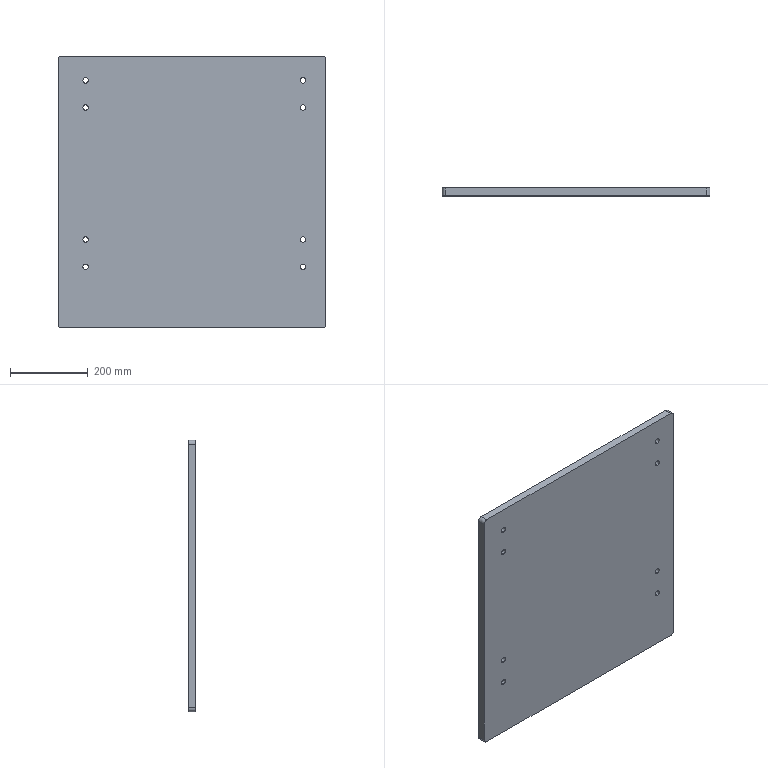Part | SolidWorks | features BaseBody 1 | 1 solid | 26 faces | box 690 x 20 x 700 mm | volume 9633653 mm3 | cylinder 20 | plane 6 | commonest cylinder face diameters 14 x16 20 x4
STEP:
#1=CARTESIAN_POINT('',(-274.,-10.,-185.5));
#2=VERTEX_POINT('',#1);
#3=CARTESIAN_POINT('',(-274.,-10.,-199.5));
#4=VERTEX_POINT('',#3);
#5=CARTESIAN_POINT('',(-274.,-10.,-192.5));
#6=DIRECTION('',(0.,-1.,0.));
#7=DIRECTION('',(0.,0.,-1.));
#8=AXIS2_PLACEMENT_3D('',#5,#6,#7);
#9=CIRCLE('',#8,7.);
#10=EDGE_CURVE('',#2,#4,#9,.T.);
#11=ORIENTED_EDGE('',*,*,#10,.T.);
#12=CARTESIAN_POINT('',(-274.,10.,-199.5));
#13=VERTEX_POINT('',#12);
#14=CARTESIAN_POINT('',(-274.,10.,-199.5));
#15=DIRECTION('',(0.,1.,0.));
#16=VECTOR('',#15,1000.);
#17=LINE('',#14,#16);
#18=EDGE_CURVE('',#4,#13,#17,.T.);
#19=ORIENTED_EDGE('',*,*,#18,.T.);
#20=CARTESIAN_POINT('',(-274.,10.,-185.5));
#21=VERTEX_POINT('',#20);
#22=CARTESIAN_POINT('',(-274.,10.,-192.5));
#23=DIRECTION('',(0.,1.,0.));
#24=DIRECTION('',(0.,0.,1.));
#25=AXIS2_PLACEMENT_3D('',#22,#23,#24);
#26=CIRCLE('',#25,7.);
#27=EDGE_CURVE('',#13,#21,#26,.T.);
#28=ORIENTED_EDGE('',*,*,#27,.T.);
#29=CARTESIAN_POINT('',(-274.,10.,-185.5));
#30=DIRECTION('',(0.,1.,0.));
#31=VECTOR('',#30,1000.);
#32=LINE('',#29,#31);
#33=EDGE_CURVE('',#2,#21,#32,.T.);
#34=ORIENTED_EDGE('',*,*,#33,.F.);
#35=EDGE_LOOP('',(#11,#19,#28,#34));
#36=FACE_OUTER_BOUND('',#35,.T.);
#37=CARTESIAN_POINT('',(-274.,10.,-192.5));
#38=DIRECTION('',(0.,1.,0.));
#39=DIRECTION('',(0.,0.,1.));
#40=AXIS2_PLACEMENT_3D('',#37,#38,#39);
#41=CYLINDRICAL_SURFACE('',#40,7.);
#42=ADVANCED_FACE('',(#36),#41,.F.);
#43=CARTESIAN_POINT('',(-274.,-10.,-115.5));
#44=VERTEX_POINT('',#43);
#45=CARTESIAN_POINT('',(-274.,-10.,-129.5));
#46=VERTEX_POINT('',#45);
#47=CARTESIAN_POINT('',(-274.,-10.,-122.5));
#48=DIRECTION('',(0.,-1.,0.));
#49=DIRECTION('',(0.,0.,-1.));
#50=AXIS2_PLACEMENT_3D('',#47,#48,#49);
#51=CIRCLE('',#50,7.);
#52=EDGE_CURVE('',#44,#46,#51,.T.);
#53=ORIENTED_EDGE('',*,*,#52,.T.);
#54=CARTESIAN_POINT('',(-274.,10.,-129.5));
#55=VERTEX_POINT('',#54);
#56=CARTESIAN_POINT('',(-274.,10.,-129.5));
#57=DIRECTION('',(0.,1.,0.));
#58=VECTOR('',#57,1000.);
#59=LINE('',#56,#58);
#60=EDGE_CURVE('',#46,#55,#59,.T.);
#61=ORIENTED_EDGE('',*,*,#60,.T.);
#62=CARTESIAN_POINT('',(-274.,10.,-115.5));
#63=VERTEX_POINT('',#62);
#64=CARTESIAN_POINT('',(-274.,10.,-122.5));
#65=DIRECTION('',(0.,1.,0.));
#66=DIRECTION('',(0.,0.,1.));
#67=AXIS2_PLACEMENT_3D('',#64,#65,#66);
#68=CIRCLE('',#67,7.);
#69=EDGE_CURVE('',#55,#63,#68,.T.);
#70=ORIENTED_EDGE('',*,*,#69,.T.);
#71=CARTESIAN_POINT('',(-274.,10.,-115.5));
#72=DIRECTION('',(0.,1.,0.));
#73=VECTOR('',#72,1000.);
#74=LINE('',#71,#73);
#75=EDGE_CURVE('',#44,#63,#74,.T.);
#76=ORIENTED_EDGE('',*,*,#75,.F.);
#77=EDGE_LOOP('',(#53,#61,#70,#76));
#78=FACE_OUTER_BOUND('',#77,.T.);
#79=CARTESIAN_POINT('',(-274.,10.,-122.5));
#80=DIRECTION('',(0.,1.,0.));
#81=DIRECTION('',(0.,0.,1.));
#82=AXIS2_PLACEMENT_3D('',#79,#80,#81);
#83=CYLINDRICAL_SURFACE('',#82,7.);
#84=ADVANCED_FACE('',(#78),#83,.F.);
#85=CARTESIAN_POINT('',(286.,-10.,-185.5));
#86=VERTEX_POINT('',#85);
#87=CARTESIAN_POINT('',(286.,-10.,-199.5));
#88=VERTEX_POINT('',#87);
#89=CARTESIAN_POINT('',(286.,-10.,-192.5));
#90=DIRECTION('',(0.,-1.,0.));
#91=DIRECTION('',(0.,0.,-1.));
#92=AXIS2_PLACEMENT_3D('',#89,#90,#91);
#93=CIRCLE('',#92,7.);
#94=EDGE_CURVE('',#86,#88,#93,.T.);
#95=ORIENTED_EDGE('',*,*,#94,.T.);
#96=CARTESIAN_POINT('',(286.,10.,-199.5));
#97=VERTEX_POINT('',#96);
#98=CARTESIAN_POINT('',(286.,10.,-199.5));
#99=DIRECTION('',(0.,1.,0.));
#100=VECTOR('',#99,1000.);
#101=LINE('',#98,#100);
#102=EDGE_CURVE('',#88,#97,#101,.T.);
#103=ORIENTED_EDGE('',*,*,#102,.T.);
#104=CARTESIAN_POINT('',(286.,10.,-185.5));
#105=VERTEX_POINT('',#104);
#106=CARTESIAN_POINT('',(286.,10.,-192.5));
#107=DIRECTION('',(0.,1.,0.));
#108=DIRECTION('',(0.,0.,1.));
#109=AXIS2_PLACEMENT_3D('',#106,#107,#108);
#110=CIRCLE('',#109,7.);
#111=EDGE_CURVE('',#97,#105,#110,.T.);
#112=ORIENTED_EDGE('',*,*,#111,.T.);
#113=CARTESIAN_POINT('',(286.,10.,-185.5));
#114=DIRECTION('',(0.,1.,0.));
#115=VECTOR('',#114,1000.);
#116=LINE('',#113,#115);
#117=EDGE_CURVE('',#86,#105,#116,.T.);
#118=ORIENTED_EDGE('',*,*,#117,.F.);
#119=EDGE_LOOP('',(#95,#103,#112,#118));
#120=FACE_OUTER_BOUND('',#119,.T.);
#121=CARTESIAN_POINT('',(286.,10.,-192.5));
#122=DIRECTION('',(0.,1.,0.));
#123=DIRECTION('',(0.,0.,1.));
#124=AXIS2_PLACEMENT_3D('',#121,#122,#123);
#125=CYLINDRICAL_SURFACE('',#124,7.);
#126=ADVANCED_FACE('',(#120),#125,.F.);
#127=CARTESIAN_POINT('',(286.,-10.,-115.5));
#128=VERTEX_POINT('',#127);
#129=CARTESIAN_POINT('',(286.,-10.,-129.5));
#130=VERTEX_POINT('',#129);
#131=CARTESIAN_POINT('',(286.,-10.,-122.5));
#132=DIRECTION('',(0.,-1.,0.));
#133=DIRECTION('',(0.,0.,-1.));
#134=AXIS2_PLACEMENT_3D('',#131,#132,#133);
#135=CIRCLE('',#134,7.);
#136=EDGE_CURVE('',#128,#130,#135,.T.);
#137=ORIENTED_EDGE('',*,*,#136,.T.);
#138=CARTESIAN_POINT('',(286.,10.,-129.5));
#139=VERTEX_POINT('',#138);
#140=CARTESIAN_POINT('',(286.,10.,-129.5));
#141=DIRECTION('',(0.,1.,0.));
#142=VECTOR('',#141,1000.);
#143=LINE('',#140,#142);
#144=EDGE_CURVE('',#130,#139,#143,.T.);
#145=ORIENTED_EDGE('',*,*,#144,.T.);
#146=CARTESIAN_POINT('',(286.,10.,-115.5));
#147=VERTEX_POINT('',#146);
#148=CARTESIAN_POINT('',(286.,10.,-122.5));
#149=DIRECTION('',(0.,1.,0.));
#150=DIRECTION('',(0.,0.,1.));
#151=AXIS2_PLACEMENT_3D('',#148,#149,#150);
#152=CIRCLE('',#151,7.);
#153=EDGE_CURVE('',#139,#147,#152,.T.);
#154=ORIENTED_EDGE('',*,*,#153,.T.);
#155=CARTESIAN_POINT('',(286.,10.,-115.5));
#156=DIRECTION('',(0.,1.,0.));
#157=VECTOR('',#156,1000.);
#158=LINE('',#155,#157);
#159=EDGE_CURVE('',#128,#147,#158,.T.);
#160=ORIENTED_EDGE('',*,*,#159,.F.);
#161=EDGE_LOOP('',(#137,#145,#154,#160));
#162=FACE_OUTER_BOUND('',#161,.T.);
#163=CARTESIAN_POINT('',(286.,10.,-122.5));
#164=DIRECTION('',(0.,1.,0.));
#165=DIRECTION('',(0.,0.,1.));
#166=AXIS2_PLACEMENT_3D('',#163,#164,#165);
#167=CYLINDRICAL_SURFACE('',#166,7.);
#168=ADVANCED_FACE('',(#162),#167,.F.);
#169=CARTESIAN_POINT('',(286.,-10.,224.5));
#170=VERTEX_POINT('',#169);
#171=CARTESIAN_POINT('',(286.,-10.,210.5));
#172=VERTEX_POINT('',#171);
#173=CARTESIAN_POINT('',(286.,-10.,217.5));
#174=DIRECTION('',(0.,-1.,0.));
#175=DIRECTION('',(0.,0.,-1.));
#176=AXIS2_PLACEMENT_3D('',#173,#174,#175);
#177=CIRCLE('',#176,7.);
#178=EDGE_CURVE('',#170,#172,#177,.T.);
#179=ORIENTED_EDGE('',*,*,#178,.T.);
#180=CARTESIAN_POINT('',(286.,10.,210.5));
#181=VERTEX_POINT('',#180);
#182=CARTESIAN_POINT('',(286.,10.,210.5));
#183=DIRECTION('',(0.,1.,0.));
#184=VECTOR('',#183,1000.);
#185=LINE('',#182,#184);
#186=EDGE_CURVE('',#172,#181,#185,.T.);
#187=ORIENTED_EDGE('',*,*,#186,.T.);
#188=CARTESIAN_POINT('',(286.,10.,224.5));
#189=VERTEX_POINT('',#188);
#190=CARTESIAN_POINT('',(286.,10.,217.5));
#191=DIRECTION('',(0.,1.,0.));
#192=DIRECTION('',(0.,0.,1.));
#193=AXIS2_PLACEMENT_3D('',#190,#191,#192);
#194=CIRCLE('',#193,7.);
#195=EDGE_CURVE('',#181,#189,#194,.T.);
#196=ORIENTED_EDGE('',*,*,#195,.T.);
#197=CARTESIAN_POINT('',(286.,10.,224.5));
#198=DIRECTION('',(0.,1.,0.));
#199=VECTOR('',#198,1000.);
#200=LINE('',#197,#199);
#201=EDGE_CURVE('',#170,#189,#200,.T.);
#202=ORIENTED_EDGE('',*,*,#201,.F.);
#203=EDGE_LOOP('',(#179,#187,#196,#202));
#204=FACE_OUTER_BOUND('',#203,.T.);
#205=CARTESIAN_POINT('',(286.,10.,217.5));
#206=DIRECTION('',(0.,1.,0.));
#207=DIRECTION('',(0.,0.,1.));
#208=AXIS2_PLACEMENT_3D('',#205,#206,#207);
#209=CYLINDRICAL_SURFACE('',#208,7.);
#210=ADVANCED_FACE('',(#204),#209,.F.);
#211=CARTESIAN_POINT('',(286.,-10.,294.5));
#212=VERTEX_POINT('',#211);
#213=CARTESIAN_POINT('',(286.,-10.,280.5));
#214=VERTEX_POINT('',#213);
#215=CARTESIAN_POINT('',(286.,-10.,287.5));
#216=DIRECTION('',(0.,-1.,0.));
#217=DIRECTION('',(0.,0.,-1.));
#218=AXIS2_PLACEMENT_3D('',#215,#216,#217);
#219=CIRCLE('',#218,7.);
#220=EDGE_CURVE('',#212,#214,#219,.T.);
#221=ORIENTED_EDGE('',*,*,#220,.T.);
#222=CARTESIAN_POINT('',(286.,10.,280.5));
#223=VERTEX_POINT('',#222);
#224=CARTESIAN_POINT('',(286.,10.,280.5));
#225=DIRECTION('',(0.,1.,0.));
#226=VECTOR('',#225,1000.);
#227=LINE('',#224,#226);
#228=EDGE_CURVE('',#214,#223,#227,.T.);
#229=ORIENTED_EDGE('',*,*,#228,.T.);
#230=CARTESIAN_POINT('',(286.,10.,294.5));
#231=VERTEX_POINT('',#230);
#232=CARTESIAN_POINT('',(286.,10.,287.5));
#233=DIRECTION('',(0.,1.,0.));
#234=DIRECTION('',(0.,0.,1.));
#235=AXIS2_PLACEMENT_3D('',#232,#233,#234);
#236=CIRCLE('',#235,7.);
#237=EDGE_CURVE('',#223,#231,#236,.T.);
#238=ORIENTED_EDGE('',*,*,#237,.T.);
#239=CARTESIAN_POINT('',(286.,10.,294.5));
#240=DIRECTION('',(0.,1.,0.));
#241=VECTOR('',#240,1000.);
#242=LINE('',#239,#241);
#243=EDGE_CURVE('',#212,#231,#242,.T.);
#244=ORIENTED_EDGE('',*,*,#243,.F.);
#245=EDGE_LOOP('',(#221,#229,#238,#244));
#246=FACE_OUTER_BOUND('',#245,.T.);
#247=CARTESIAN_POINT('',(286.,10.,287.5));
#248=DIRECTION('',(0.,1.,0.));
#249=DIRECTION('',(0.,0.,1.));
#250=AXIS2_PLACEMENT_3D('',#247,#248,#249);
#251=CYLINDRICAL_SURFACE('',#250,7.);
#252=ADVANCED_FACE('',(#246),#251,.F.);
#253=CARTESIAN_POINT('',(-274.,-10.,224.5));
#254=VERTEX_POINT('',#253);
#255=CARTESIAN_POINT('',(-274.,-10.,210.5));
#256=VERTEX_POINT('',#255);
#257=CARTESIAN_POINT('',(-274.,-10.,217.5));
#258=DIRECTION('',(0.,-1.,0.));
#259=DIRECTION('',(0.,0.,-1.));
#260=AXIS2_PLACEMENT_3D('',#257,#258,#259);
#261=CIRCLE('',#260,7.);
#262=EDGE_CURVE('',#254,#256,#261,.T.);
#263=ORIENTED_EDGE('',*,*,#262,.T.);
#264=CARTESIAN_POINT('',(-274.,10.,210.5));
#265=VERTEX_POINT('',#264);
#266=CARTESIAN_POINT('',(-274.,10.,210.5));
#267=DIRECTION('',(0.,1.,0.));
#268=VECTOR('',#267,1000.);
#269=LINE('',#266,#268);
#270=EDGE_CURVE('',#256,#265,#269,.T.);
#271=ORIENTED_EDGE('',*,*,#270,.T.);
#272=CARTESIAN_POINT('',(-274.,10.,224.5));
#273=VERTEX_POINT('',#272);
#274=CARTESIAN_POINT('',(-274.,10.,217.5));
#275=DIRECTION('',(0.,1.,0.));
#276=DIRECTION('',(0.,0.,1.));
#277=AXIS2_PLACEMENT_3D('',#274,#275,#276);
#278=CIRCLE('',#277,7.);
#279=EDGE_CURVE('',#265,#273,#278,.T.);
#280=ORIENTED_EDGE('',*,*,#279,.T.);
#281=CARTESIAN_POINT('',(-274.,10.,224.5));
#282=DIRECTION('',(0.,1.,0.));
#283=VECTOR('',#282,1000.);
#284=LINE('',#281,#283);
#285=EDGE_CURVE('',#254,#273,#284,.T.);
#286=ORIENTED_EDGE('',*,*,#285,.F.);
#287=EDGE_LOOP('',(#263,#271,#280,#286));
#288=FACE_OUTER_BOUND('',#287,.T.);
#289=CARTESIAN_POINT('',(-274.,10.,217.5));
#290=DIRECTION('',(0.,1.,0.));
#291=DIRECTION('',(0.,0.,1.));
#292=AXIS2_PLACEMENT_3D('',#289,#290,#291);
#293=CYLINDRICAL_SURFACE('',#292,7.);
#294=ADVANCED_FACE('',(#288),#293,.F.);
#295=CARTESIAN_POINT('',(-274.,-10.,294.5));
#296=VERTEX_POINT('',#295);
#297=CARTESIAN_POINT('',(-274.,-10.,280.5));
#298=VERTEX_POINT('',#297);
#299=CARTESIAN_POINT('',(-274.,-10.,287.5));
#300=DIRECTION('',(0.,-1.,0.));
#301=DIRECTION('',(0.,0.,-1.));
#302=AXIS2_PLACEMENT_3D('',#299,#300,#301);
#303=CIRCLE('',#302,7.);
#304=EDGE_CURVE('',#296,#298,#303,.T.);
#305=ORIENTED_EDGE('',*,*,#304,.T.);
#306=CARTESIAN_POINT('',(-274.,10.,280.5));
#307=VERTEX_POINT('',#306);
#308=CARTESIAN_POINT('',(-274.,10.,280.5));
#309=DIRECTION('',(0.,1.,0.));
#310=VECTOR('',#309,1000.);
#311=LINE('',#308,#310);
#312=EDGE_CURVE('',#298,#307,#311,.T.);
#313=ORIENTED_EDGE('',*,*,#312,.T.);
#314=CARTESIAN_POINT('',(-274.,10.,294.5));
#315=VERTEX_POINT('',#314);
#316=CARTESIAN_POINT('',(-274.,10.,287.5));
#317=DIRECTION('',(0.,1.,0.));
#318=DIRECTION('',(0.,0.,1.));
#319=AXIS2_PLACEMENT_3D('',#316,#317,#318);
#320=CIRCLE('',#319,7.);
#321=EDGE_CURVE('',#307,#315,#320,.T.);
#322=ORIENTED_EDGE('',*,*,#321,.T.);
#323=CARTESIAN_POINT('',(-274.,10.,294.5));
#324=DIRECTION('',(0.,1.,0.));
#325=VECTOR('',#324,1000.);
#326=LINE('',#323,#325);
#327=EDGE_CURVE('',#296,#315,#326,.T.);
#328=ORIENTED_EDGE('',*,*,#327,.F.);
#329=EDGE_LOOP('',(#305,#313,#322,#328));
#330=FACE_OUTER_BOUND('',#329,.T.);
#331=CARTESIAN_POINT('',(-274.,10.,287.5));
#332=DIRECTION('',(0.,1.,0.));
#333=DIRECTION('',(0.,0.,1.));
#334=AXIS2_PLACEMENT_3D('',#331,#332,#333);
#335=CYLINDRICAL_SURFACE('',#334,7.);
#336=ADVANCED_FACE('',(#330),#335,.F.);
#337=CARTESIAN_POINT('',(345.,-10.,-340.));
#338=VERTEX_POINT('',#337);
#339=CARTESIAN_POINT('',(335.,-10.,-350.));
#340=VERTEX_POINT('',#339);
#341=CARTESIAN_POINT('',(335.,-10.,-340.));
#342=DIRECTION('',(0.,1.,0.));
#343=DIRECTION('',(0.,0.,-1.));
#344=AXIS2_PLACEMENT_3D('',#341,#342,#343);
#345=CIRCLE('',#344,10.);
#346=EDGE_CURVE('',#338,#340,#345,.T.);
#347=ORIENTED_EDGE('',*,*,#346,.T.);
#348=CARTESIAN_POINT('',(335.,10.,-350.));
#349=VERTEX_POINT('',#348);
#350=CARTESIAN_POINT('',(335.,10.,-350.));
#351=DIRECTION('',(0.,-1.,0.));
#352=VECTOR('',#351,1000.);
#353=LINE('',#350,#352);
#354=EDGE_CURVE('',#349,#340,#353,.T.);
#355=ORIENTED_EDGE('',*,*,#354,.F.);
#356=CARTESIAN_POINT('',(345.,10.,-340.));
#357=VERTEX_POINT('',#356);
#358=CARTESIAN_POINT('',(335.,10.,-340.));
#359=DIRECTION('',(0.,1.,0.));
#360=DIRECTION('',(0.,0.,-1.));
#361=AXIS2_PLACEMENT_3D('',#358,#359,#360);
#362=CIRCLE('',#361,10.);
#363=EDGE_CURVE('',#357,#349,#362,.T.);
#364=ORIENTED_EDGE('',*,*,#363,.F.);
#365=CARTESIAN_POINT('',(345.,10.,-340.));
#366=DIRECTION('',(0.,-1.,0.));
#367=VECTOR('',#366,1000.);
#368=LINE('',#365,#367);
#369=EDGE_CURVE('',#357,#338,#368,.T.);
#370=ORIENTED_EDGE('',*,*,#369,.T.);
#371=EDGE_LOOP('',(#347,#355,#364,#370));
#372=FACE_OUTER_BOUND('',#371,.T.);
#373=CARTESIAN_POINT('',(335.,10.,-340.));
#374=DIRECTION('',(0.,-1.,0.));
#375=DIRECTION('',(0.,0.,-1.));
#376=AXIS2_PLACEMENT_3D('',#373,#374,#375);
#377=CYLINDRICAL_SURFACE('',#376,10.);
#378=ADVANCED_FACE('',(#372),#377,.T.);
#379=CARTESIAN_POINT('',(-335.,-10.,-350.));
#380=VERTEX_POINT('',#379);
#381=CARTESIAN_POINT('',(-335.,-10.,-350.));
#382=DIRECTION('',(-1.,0.,0.));
#383=VECTOR('',#382,1000.);
#384=LINE('',#381,#383);
#385=EDGE_CURVE('',#340,#380,#384,.T.);
#386=ORIENTED_EDGE('',*,*,#385,.T.);
#387=CARTESIAN_POINT('',(-335.,10.,-350.));
#388=VERTEX_POINT('',#387);
#389=CARTESIAN_POINT('',(-335.,10.,-350.));
#390=DIRECTION('',(0.,-1.,0.));
#391=VECTOR('',#390,1000.);
#392=LINE('',#389,#391);
#393=EDGE_CURVE('',#388,#380,#392,.T.);
#394=ORIENTED_EDGE('',*,*,#393,.F.);
#395=CARTESIAN_POINT('',(-335.,10.,-350.));
#396=DIRECTION('',(-1.,0.,0.));
#397=VECTOR('',#396,1000.);
#398=LINE('',#395,#397);
#399=EDGE_CURVE('',#349,#388,#398,.T.);
#400=ORIENTED_EDGE('',*,*,#399,.F.);
#401=ORIENTED_EDGE('',*,*,#354,.T.);
#402=EDGE_LOOP('',(#386,#394,#400,#401));
#403=FACE_OUTER_BOUND('',#402,.T.);
#404=CARTESIAN_POINT('',(-335.,10.,-350.));
#405=DIRECTION('',(0.,0.,1.));
#406=DIRECTION('',(1.,0.,0.));
#407=AXIS2_PLACEMENT_3D('',#404,#405,#406);
#408=PLANE('',#407);
#409=ADVANCED_FACE('',(#403),#408,.F.);
#410=CARTESIAN_POINT('',(-345.,-10.,-340.));
#411=VERTEX_POINT('',#410);
#412=CARTESIAN_POINT('',(-335.,-10.,-340.));
#413=DIRECTION('',(0.,1.,0.));
#414=DIRECTION('',(0.,0.,1.));
#415=AXIS2_PLACEMENT_3D('',#412,#413,#414);
#416=CIRCLE('',#415,10.);
#417=EDGE_CURVE('',#380,#411,#416,.T.);
#418=ORIENTED_EDGE('',*,*,#417,.T.);
#419=CARTESIAN_POINT('',(-345.,10.,-340.));
#420=VERTEX_POINT('',#419);
#421=CARTESIAN_POINT('',(-345.,10.,-340.));
#422=DIRECTION('',(0.,-1.,0.));
#423=VECTOR('',#422,1000.);
#424=LINE('',#421,#423);
#425=EDGE_CURVE('',#420,#411,#424,.T.);
#426=ORIENTED_EDGE('',*,*,#425,.F.);
#427=CARTESIAN_POINT('',(-335.,10.,-340.));
#428=DIRECTION('',(0.,1.,0.));
#429=DIRECTION('',(0.,0.,1.));
#430=AXIS2_PLACEMENT_3D('',#427,#428,#429);
#431=CIRCLE('',#430,10.);
#432=EDGE_CURVE('',#388,#420,#431,.T.);
#433=ORIENTED_EDGE('',*,*,#432,.F.);
#434=ORIENTED_EDGE('',*,*,#393,.T.);
#435=EDGE_LOOP('',(#418,#426,#433,#434));
#436=FACE_OUTER_BOUND('',#435,.T.);
#437=CARTESIAN_POINT('',(-335.,10.,-340.));
#438=DIRECTION('',(0.,-1.,0.));
#439=DIRECTION('',(0.,0.,-1.));
#440=AXIS2_PLACEMENT_3D('',#437,#438,#439);
#441=CYLINDRICAL_SURFACE('',#440,10.);
#442=ADVANCED_FACE('',(#436),#441,.T.);
#443=CARTESIAN_POINT('',(-345.,-10.,340.));
#444=VERTEX_POINT('',#443);
#445=CARTESIAN_POINT('',(-345.,-10.,-340.));
#446=DIRECTION('',(0.,0.,1.));
#447=VECTOR('',#446,1000.);
#448=LINE('',#445,#447);
#449=EDGE_CURVE('',#411,#444,#448,.T.);
#450=ORIENTED_EDGE('',*,*,#449,.T.);
#451=CARTESIAN_POINT('',(-345.,10.,340.));
#452=VERTEX_POINT('',#451);
#453=CARTESIAN_POINT('',(-345.,10.,340.));
#454=DIRECTION('',(0.,-1.,0.));
#455=VECTOR('',#454,1000.);
#456=LINE('',#453,#455);
#457=EDGE_CURVE('',#452,#444,#456,.T.);
#458=ORIENTED_EDGE('',*,*,#457,.F.);
#459=CARTESIAN_POINT('',(-345.,10.,-340.));
#460=DIRECTION('',(0.,0.,1.));
#461=VECTOR('',#460,1000.);
#462=LINE('',#459,#461);
#463=EDGE_CURVE('',#420,#452,#462,.T.);
#464=ORIENTED_EDGE('',*,*,#463,.F.);
#465=ORIENTED_EDGE('',*,*,#425,.T.);
#466=EDGE_LOOP('',(#450,#458,#464,#465));
#467=FACE_OUTER_BOUND('',#466,.T.);
#468=CARTESIAN_POINT('',(-345.,10.,-340.));
#469=DIRECTION('',(1.,0.,0.));
#470=DIRECTION('',(0.,0.,-1.));
#471=AXIS2_PLACEMENT_3D('',#468,#469,#470);
#472=PLANE('',#471);
#473=ADVANCED_FACE('',(#467),#472,.F.);
#474=CARTESIAN_POINT('',(-335.,-10.,350.));
#475=VERTEX_POINT('',#474);
#476=CARTESIAN_POINT('',(-335.,-10.,340.));
#477=DIRECTION('',(0.,1.,0.));
#478=DIRECTION('',(0.,0.,1.));
#479=AXIS2_PLACEMENT_3D('',#476,#477,#478);
#480=CIRCLE('',#479,10.);
#481=EDGE_CURVE('',#444,#475,#480,.T.);
#482=ORIENTED_EDGE('',*,*,#481,.T.);
#483=CARTESIAN_POINT('',(-335.,10.,350.));
#484=VERTEX_POINT('',#483);
#485=CARTESIAN_POINT('',(-335.,10.,350.));
#486=DIRECTION('',(0.,-1.,0.));
#487=VECTOR('',#486,1000.);
#488=LINE('',#485,#487);
#489=EDGE_CURVE('',#484,#475,#488,.T.);
#490=ORIENTED_EDGE('',*,*,#489,.F.);
#491=CARTESIAN_POINT('',(-335.,10.,340.));
#492=DIRECTION('',(0.,1.,0.));
#493=DIRECTION('',(0.,0.,1.));
#494=AXIS2_PLACEMENT_3D('',#491,#492,#493);
#495=CIRCLE('',#494,10.);
#496=EDGE_CURVE('',#452,#484,#495,.T.);
#497=ORIENTED_EDGE('',*,*,#496,.F.);
#498=ORIENTED_EDGE('',*,*,#457,.T.);
#499=EDGE_LOOP('',(#482,#490,#497,#498));
#500=FACE_OUTER_BOUND('',#499,.T.);
#501=CARTESIAN_POINT('',(-335.,10.,340.));
#502=DIRECTION('',(0.,-1.,0.));
#503=DIRECTION('',(0.,0.,-1.));
#504=AXIS2_PLACEMENT_3D('',#501,#502,#503);
#505=CYLINDRICAL_SURFACE('',#504,10.);
#506=ADVANCED_FACE('',(#500),#505,.T.);
#507=CARTESIAN_POINT('',(335.,-10.,350.));
#508=VERTEX_POINT('',#507);
#509=CARTESIAN_POINT('',(-335.,-10.,350.));
#510=DIRECTION('',(1.,0.,0.));
#511=VECTOR('',#510,1000.);
#512=LINE('',#509,#511);
#513=EDGE_CURVE('',#475,#508,#512,.T.);
#514=ORIENTED_EDGE('',*,*,#513,.T.);
#515=CARTESIAN_POINT('',(335.,10.,350.));
#516=VERTEX_POINT('',#515);
#517=CARTESIAN_POINT('',(335.,10.,350.));
#518=DIRECTION('',(0.,-1.,0.));
#519=VECTOR('',#518,1000.);
#520=LINE('',#517,#519);
#521=EDGE_CURVE('',#516,#508,#520,.T.);
#522=ORIENTED_EDGE('',*,*,#521,.F.);
#523=CARTESIAN_POINT('',(-335.,10.,350.));
#524=DIRECTION('',(1.,0.,0.));
#525=VECTOR('',#524,1000.);
#526=LINE('',#523,#525);
#527=EDGE_CURVE('',#484,#516,#526,.T.);
#528=ORIENTED_EDGE('',*,*,#527,.F.);
#529=ORIENTED_EDGE('',*,*,#489,.T.);
#530=EDGE_LOOP('',(#514,#522,#528,#529));
#531=FACE_OUTER_BOUND('',#530,.T.);
#532=CARTESIAN_POINT('',(-335.,10.,350.));
#533=DIRECTION('',(0.,0.,-1.));
#534=DIRECTION('',(-1.,0.,0.));
#535=AXIS2_PLACEMENT_3D('',#532,#533,#534);
#536=PLANE('',#535);
#537=ADVANCED_FACE('',(#531),#536,.F.);
#538=CARTESIAN_POINT('',(345.,-10.,340.));
#539=VERTEX_POINT('',#538);
#540=CARTESIAN_POINT('',(335.,-10.,340.));
#541=DIRECTION('',(0.,1.,0.));
#542=DIRECTION('',(0.,0.,1.));
#543=AXIS2_PLACEMENT_3D('',#540,#541,#542);
#544=CIRCLE('',#543,10.);
#545=EDGE_CURVE('',#508,#539,#544,.T.);
#546=ORIENTED_EDGE('',*,*,#545,.T.);
#547=CARTESIAN_POINT('',(345.,10.,340.));
#548=VERTEX_POINT('',#547);
#549=CARTESIAN_POINT('',(345.,10.,340.));
#550=DIRECTION('',(0.,-1.,0.));
#551=VECTOR('',#550,1000.);
#552=LINE('',#549,#551);
#553=EDGE_CURVE('',#548,#539,#552,.T.);
#554=ORIENTED_EDGE('',*,*,#553,.F.);
#555=CARTESIAN_POINT('',(335.,10.,340.));
#556=DIRECTION('',(0.,1.,0.));
#557=DIRECTION('',(0.,0.,1.));
#558=AXIS2_PLACEMENT_3D('',#555,#556,#557);
#559=CIRCLE('',#558,10.);
#560=EDGE_CURVE('',#516,#548,#559,.T.);
#561=ORIENTED_EDGE('',*,*,#560,.F.);
#562=ORIENTED_EDGE('',*,*,#521,.T.);
#563=EDGE_LOOP('',(#546,#554,#561,#562));
#564=FACE_OUTER_BOUND('',#563,.T.);
#565=CARTESIAN_POINT('',(335.,10.,340.));
#566=DIRECTION('',(0.,-1.,0.));
#567=DIRECTION('',(0.,0.,-1.));
#568=AXIS2_PLACEMENT_3D('',#565,#566,#567);
#569=CYLINDRICAL_SURFACE('',#568,10.);
#570=ADVANCED_FACE('',(#564),#569,.T.);
#571=CARTESIAN_POINT('',(345.,-10.,-340.));
#572=DIRECTION('',(0.,0.,-1.));
#573=VECTOR('',#572,1000.);
#574=LINE('',#571,#573);
#575=EDGE_CURVE('',#539,#338,#574,.T.);
#576=ORIENTED_EDGE('',*,*,#575,.T.);
#577=ORIENTED_EDGE('',*,*,#369,.F.);
#578=CARTESIAN_POINT('',(345.,10.,-340.));
#579=DIRECTION('',(0.,0.,-1.));
#580=VECTOR('',#579,1000.);
#581=LINE('',#578,#580);
#582=EDGE_CURVE('',#548,#357,#581,.T.);
#583=ORIENTED_EDGE('',*,*,#582,.F.);
#584=ORIENTED_EDGE('',*,*,#553,.T.);
#585=EDGE_LOOP('',(#576,#577,#583,#584));
#586=FACE_OUTER_BOUND('',#585,.T.);
#587=CARTESIAN_POINT('',(345.,10.,-340.));
#588=DIRECTION('',(-1.,0.,0.));
#589=DIRECTION('',(0.,0.,1.));
#590=AXIS2_PLACEMENT_3D('',#587,#588,#589);
#591=PLANE('',#590);
#592=ADVANCED_FACE('',(#586),#591,.F.);
#593=CARTESIAN_POINT('',(-274.,10.,-192.5));
#594=DIRECTION('',(0.,1.,0.));
#595=DIRECTION('',(0.,0.,1.));
#596=AXIS2_PLACEMENT_3D('',#593,#594,#595);
#597=CIRCLE('',#596,7.);
#598=EDGE_CURVE('',#21,#13,#597,.T.);
#599=ORIENTED_EDGE('',*,*,#598,.F.);
#600=ORIENTED_EDGE('',*,*,#27,.F.);
#601=EDGE_LOOP('',(#599,#600));
#602=FACE_BOUND('',#601,.T.);
#603=CARTESIAN_POINT('',(-274.,10.,-122.5));
#604=DIRECTION('',(0.,1.,0.));
#605=DIRECTION('',(0.,0.,1.));
#606=AXIS2_PLACEMENT_3D('',#603,#604,#605);
#607=CIRCLE('',#606,7.);
#608=EDGE_CURVE('',#63,#55,#607,.T.);
#609=ORIENTED_EDGE('',*,*,#608,.F.);
#610=ORIENTED_EDGE('',*,*,#69,.F.);
#611=EDGE_LOOP('',(#609,#610));
#612=FACE_BOUND('',#611,.T.);
#613=CARTESIAN_POINT('',(286.,10.,-192.5));
#614=DIRECTION('',(0.,1.,0.));
#615=DIRECTION('',(0.,0.,1.));
#616=AXIS2_PLACEMENT_3D('',#613,#614,#615);
#617=CIRCLE('',#616,7.);
#618=EDGE_CURVE('',#105,#97,#617,.T.);
#619=ORIENTED_EDGE('',*,*,#618,.F.);
#620=ORIENTED_EDGE('',*,*,#111,.F.);
#621=EDGE_LOOP('',(#619,#620));
#622=FACE_BOUND('',#621,.T.);
#623=CARTESIAN_POINT('',(286.,10.,-122.5));
#624=DIRECTION('',(0.,1.,0.));
#625=DIRECTION('',(0.,0.,1.));
#626=AXIS2_PLACEMENT_3D('',#623,#624,#625);
#627=CIRCLE('',#626,7.);
#628=EDGE_CURVE('',#147,#139,#627,.T.);
#629=ORIENTED_EDGE('',*,*,#628,.F.);
#630=ORIENTED_EDGE('',*,*,#153,.F.);
#631=EDGE_LOOP('',(#629,#630));
#632=FACE_BOUND('',#631,.T.);
#633=CARTESIAN_POINT('',(286.,10.,217.5));
#634=DIRECTION('',(0.,1.,0.));
#635=DIRECTION('',(0.,0.,1.));
#636=AXIS2_PLACEMENT_3D('',#633,#634,#635);
#637=CIRCLE('',#636,7.);
#638=EDGE_CURVE('',#189,#181,#637,.T.);
#639=ORIENTED_EDGE('',*,*,#638,.F.);
#640=ORIENTED_EDGE('',*,*,#195,.F.);
#641=EDGE_LOOP('',(#639,#640));
#642=FACE_BOUND('',#641,.T.);
#643=CARTESIAN_POINT('',(286.,10.,287.5));
#644=DIRECTION('',(0.,1.,0.));
#645=DIRECTION('',(0.,0.,1.));
#646=AXIS2_PLACEMENT_3D('',#643,#644,#645);
#647=CIRCLE('',#646,7.);
#648=EDGE_CURVE('',#231,#223,#647,.T.);
#649=ORIENTED_EDGE('',*,*,#648,.F.);
#650=ORIENTED_EDGE('',*,*,#237,.F.);
#651=EDGE_LOOP('',(#649,#650));
#652=FACE_BOUND('',#651,.T.);
#653=CARTESIAN_POINT('',(-274.,10.,217.5));
#654=DIRECTION('',(0.,1.,0.));
#655=DIRECTION('',(0.,0.,1.));
#656=AXIS2_PLACEMENT_3D('',#653,#654,#655);
#657=CIRCLE('',#656,7.);
#658=EDGE_CURVE('',#273,#265,#657,.T.);
#659=ORIENTED_EDGE('',*,*,#658,.F.);
#660=ORIENTED_EDGE('',*,*,#279,.F.);
#661=EDGE_LOOP('',(#659,#660));
#662=FACE_BOUND('',#661,.T.);
#663=CARTESIAN_POINT('',(-274.,10.,287.5));
#664=DIRECTION('',(0.,1.,0.));
#665=DIRECTION('',(0.,0.,1.));
#666=AXIS2_PLACEMENT_3D('',#663,#664,#665);
#667=CIRCLE('',#666,7.);
#668=EDGE_CURVE('',#315,#307,#667,.T.);
#669=ORIENTED_EDGE('',*,*,#668,.F.);
#670=ORIENTED_EDGE('',*,*,#321,.F.);
#671=EDGE_LOOP('',(#669,#670));
#672=FACE_BOUND('',#671,.T.);
#673=ORIENTED_EDGE('',*,*,#363,.T.);
#674=ORIENTED_EDGE('',*,*,#399,.T.);
#675=ORIENTED_EDGE('',*,*,#432,.T.);
#676=ORIENTED_EDGE('',*,*,#463,.T.);
#677=ORIENTED_EDGE('',*,*,#496,.T.);
#678=ORIENTED_EDGE('',*,*,#527,.T.);
#679=ORIENTED_EDGE('',*,*,#560,.T.);
#680=ORIENTED_EDGE('',*,*,#582,.T.);
#681=EDGE_LOOP('',(#673,#674,#675,#676,#677,#678,#679,#680));
#682=FACE_OUTER_BOUND('',#681,.T.);
#683=CARTESIAN_POINT('',(335.,10.,-340.));
#684=DIRECTION('',(0.,-1.,0.));
#685=DIRECTION('',(0.,0.,-1.));
#686=AXIS2_PLACEMENT_3D('',#683,#684,#685);
#687=PLANE('',#686);
#688=ADVANCED_FACE('',(#602,#612,#622,#632,#642,#652,#662,#672,#682),#687,.F.);
#689=ORIENTED_EDGE('',*,*,#10,.F.);
#690=CARTESIAN_POINT('',(-274.,-10.,-192.5));
#691=DIRECTION('',(0.,-1.,0.));
#692=DIRECTION('',(0.,0.,-1.));
#693=AXIS2_PLACEMENT_3D('',#690,#691,#692);
#694=CIRCLE('',#693,7.);
#695=EDGE_CURVE('',#4,#2,#694,.T.);
#696=ORIENTED_EDGE('',*,*,#695,.F.);
#697=EDGE_LOOP('',(#689,#696));
#698=FACE_BOUND('',#697,.T.);
#699=ORIENTED_EDGE('',*,*,#52,.F.);
#700=CARTESIAN_POINT('',(-274.,-10.,-122.5));
#701=DIRECTION('',(0.,-1.,0.));
#702=DIRECTION('',(0.,0.,-1.));
#703=AXIS2_PLACEMENT_3D('',#700,#701,#702);
#704=CIRCLE('',#703,7.);
#705=EDGE_CURVE('',#46,#44,#704,.T.);
#706=ORIENTED_EDGE('',*,*,#705,.F.);
#707=EDGE_LOOP('',(#699,#706));
#708=FACE_BOUND('',#707,.T.);
#709=ORIENTED_EDGE('',*,*,#94,.F.);
#710=CARTESIAN_POINT('',(286.,-10.,-192.5));
#711=DIRECTION('',(0.,-1.,0.));
#712=DIRECTION('',(0.,0.,-1.));
#713=AXIS2_PLACEMENT_3D('',#710,#711,#712);
#714=CIRCLE('',#713,7.);
#715=EDGE_CURVE('',#88,#86,#714,.T.);
#716=ORIENTED_EDGE('',*,*,#715,.F.);
#717=EDGE_LOOP('',(#709,#716));
#718=FACE_BOUND('',#717,.T.);
#719=ORIENTED_EDGE('',*,*,#136,.F.);
#720=CARTESIAN_POINT('',(286.,-10.,-122.5));
#721=DIRECTION('',(0.,-1.,0.));
#722=DIRECTION('',(0.,0.,-1.));
#723=AXIS2_PLACEMENT_3D('',#720,#721,#722);
#724=CIRCLE('',#723,7.);
#725=EDGE_CURVE('',#130,#128,#724,.T.);
#726=ORIENTED_EDGE('',*,*,#725,.F.);
#727=EDGE_LOOP('',(#719,#726));
#728=FACE_BOUND('',#727,.T.);
#729=ORIENTED_EDGE('',*,*,#178,.F.);
#730=CARTESIAN_POINT('',(286.,-10.,217.5));
#731=DIRECTION('',(0.,-1.,0.));
#732=DIRECTION('',(0.,0.,-1.));
#733=AXIS2_PLACEMENT_3D('',#730,#731,#732);
#734=CIRCLE('',#733,7.);
#735=EDGE_CURVE('',#172,#170,#734,.T.);
#736=ORIENTED_EDGE('',*,*,#735,.F.);
#737=EDGE_LOOP('',(#729,#736));
#738=FACE_BOUND('',#737,.T.);
#739=ORIENTED_EDGE('',*,*,#220,.F.);
#740=CARTESIAN_POINT('',(286.,-10.,287.5));
#741=DIRECTION('',(0.,-1.,0.));
#742=DIRECTION('',(0.,0.,-1.));
#743=AXIS2_PLACEMENT_3D('',#740,#741,#742);
#744=CIRCLE('',#743,7.);
#745=EDGE_CURVE('',#214,#212,#744,.T.);
#746=ORIENTED_EDGE('',*,*,#745,.F.);
#747=EDGE_LOOP('',(#739,#746));
#748=FACE_BOUND('',#747,.T.);
#749=ORIENTED_EDGE('',*,*,#262,.F.);
#750=CARTESIAN_POINT('',(-274.,-10.,217.5));
#751=DIRECTION('',(0.,-1.,0.));
#752=DIRECTION('',(0.,0.,-1.));
#753=AXIS2_PLACEMENT_3D('',#750,#751,#752);
#754=CIRCLE('',#753,7.);
#755=EDGE_CURVE('',#256,#254,#754,.T.);
#756=ORIENTED_EDGE('',*,*,#755,.F.);
#757=EDGE_LOOP('',(#749,#756));
#758=FACE_BOUND('',#757,.T.);
#759=ORIENTED_EDGE('',*,*,#304,.F.);
#760=CARTESIAN_POINT('',(-274.,-10.,287.5));
#761=DIRECTION('',(0.,-1.,0.));
#762=DIRECTION('',(0.,0.,-1.));
#763=AXIS2_PLACEMENT_3D('',#760,#761,#762);
#764=CIRCLE('',#763,7.);
#765=EDGE_CURVE('',#298,#296,#764,.T.);
#766=ORIENTED_EDGE('',*,*,#765,.F.);
#767=EDGE_LOOP('',(#759,#766));
#768=FACE_BOUND('',#767,.T.);
#769=ORIENTED_EDGE('',*,*,#346,.F.);
#770=ORIENTED_EDGE('',*,*,#575,.F.);
#771=ORIENTED_EDGE('',*,*,#545,.F.);
#772=ORIENTED_EDGE('',*,*,#513,.F.);
#773=ORIENTED_EDGE('',*,*,#481,.F.);
#774=ORIENTED_EDGE('',*,*,#449,.F.);
#775=ORIENTED_EDGE('',*,*,#417,.F.);
#776=ORIENTED_EDGE('',*,*,#385,.F.);
#777=EDGE_LOOP('',(#769,#770,#771,#772,#773,#774,#775,#776));
#778=FACE_OUTER_BOUND('',#777,.T.);
#779=CARTESIAN_POINT('',(335.,-10.,-340.));
#780=DIRECTION('',(0.,-1.,0.));
#781=DIRECTION('',(0.,0.,-1.));
#782=AXIS2_PLACEMENT_3D('',#779,#780,#781);
#783=PLANE('',#782);
#784=ADVANCED_FACE('',(#698,#708,#718,#728,#738,#748,#758,#768,#778),#783,.T.);
#785=ORIENTED_EDGE('',*,*,#312,.F.);
#786=ORIENTED_EDGE('',*,*,#765,.T.);
#787=ORIENTED_EDGE('',*,*,#327,.T.);
#788=ORIENTED_EDGE('',*,*,#668,.T.);
#789=EDGE_LOOP('',(#785,#786,#787,#788));
#790=FACE_OUTER_BOUND('',#789,.T.);
#791=CARTESIAN_POINT('',(-274.,10.,287.5));
#792=DIRECTION('',(0.,1.,0.));
#793=DIRECTION('',(0.,0.,1.));
#794=AXIS2_PLACEMENT_3D('',#791,#792,#793);
#795=CYLINDRICAL_SURFACE('',#794,7.);
#796=ADVANCED_FACE('',(#790),#795,.F.);
#797=ORIENTED_EDGE('',*,*,#270,.F.);
#798=ORIENTED_EDGE('',*,*,#755,.T.);
#799=ORIENTED_EDGE('',*,*,#285,.T.);
#800=ORIENTED_EDGE('',*,*,#658,.T.);
#801=EDGE_LOOP('',(#797,#798,#799,#800));
#802=FACE_OUTER_BOUND('',#801,.T.);
#803=CARTESIAN_POINT('',(-274.,10.,217.5));
#804=DIRECTION('',(0.,1.,0.));
#805=DIRECTION('',(0.,0.,1.));
#806=AXIS2_PLACEMENT_3D('',#803,#804,#805);
#807=CYLINDRICAL_SURFACE('',#806,7.);
#808=ADVANCED_FACE('',(#802),#807,.F.);
#809=ORIENTED_EDGE('',*,*,#228,.F.);
#810=ORIENTED_EDGE('',*,*,#745,.T.);
#811=ORIENTED_EDGE('',*,*,#243,.T.);
#812=ORIENTED_EDGE('',*,*,#648,.T.);
#813=EDGE_LOOP('',(#809,#810,#811,#812));
#814=FACE_OUTER_BOUND('',#813,.T.);
#815=CARTESIAN_POINT('',(286.,10.,287.5));
#816=DIRECTION('',(0.,1.,0.));
#817=DIRECTION('',(0.,0.,1.));
#818=AXIS2_PLACEMENT_3D('',#815,#816,#817);
#819=CYLINDRICAL_SURFACE('',#818,7.);
#820=ADVANCED_FACE('',(#814),#819,.F.);
#821=ORIENTED_EDGE('',*,*,#186,.F.);
#822=ORIENTED_EDGE('',*,*,#735,.T.);
#823=ORIENTED_EDGE('',*,*,#201,.T.);
#824=ORIENTED_EDGE('',*,*,#638,.T.);
#825=EDGE_LOOP('',(#821,#822,#823,#824));
#826=FACE_OUTER_BOUND('',#825,.T.);
#827=CARTESIAN_POINT('',(286.,10.,217.5));
#828=DIRECTION('',(0.,1.,0.));
#829=DIRECTION('',(0.,0.,1.));
#830=AXIS2_PLACEMENT_3D('',#827,#828,#829);
#831=CYLINDRICAL_SURFACE('',#830,7.);
#832=ADVANCED_FACE('',(#826),#831,.F.);
#833=ORIENTED_EDGE('',*,*,#144,.F.);
#834=ORIENTED_EDGE('',*,*,#725,.T.);
#835=ORIENTED_EDGE('',*,*,#159,.T.);
#836=ORIENTED_EDGE('',*,*,#628,.T.);
#837=EDGE_LOOP('',(#833,#834,#835,#836));
#838=FACE_OUTER_BOUND('',#837,.T.);
#839=CARTESIAN_POINT('',(286.,10.,-122.5));
#840=DIRECTION('',(0.,1.,0.));
#841=DIRECTION('',(0.,0.,1.));
#842=AXIS2_PLACEMENT_3D('',#839,#840,#841);
#843=CYLINDRICAL_SURFACE('',#842,7.);
#844=ADVANCED_FACE('',(#838),#843,.F.);
#845=ORIENTED_EDGE('',*,*,#102,.F.);
#846=ORIENTED_EDGE('',*,*,#715,.T.);
#847=ORIENTED_EDGE('',*,*,#117,.T.);
#848=ORIENTED_EDGE('',*,*,#618,.T.);
#849=EDGE_LOOP('',(#845,#846,#847,#848));
#850=FACE_OUTER_BOUND('',#849,.T.);
#851=CARTESIAN_POINT('',(286.,10.,-192.5));
#852=DIRECTION('',(0.,1.,0.));
#853=DIRECTION('',(0.,0.,1.));
#854=AXIS2_PLACEMENT_3D('',#851,#852,#853);
#855=CYLINDRICAL_SURFACE('',#854,7.);
#856=ADVANCED_FACE('',(#850),#855,.F.);
#857=ORIENTED_EDGE('',*,*,#60,.F.);
#858=ORIENTED_EDGE('',*,*,#705,.T.);
#859=ORIENTED_EDGE('',*,*,#75,.T.);
#860=ORIENTED_EDGE('',*,*,#608,.T.);
#861=EDGE_LOOP('',(#857,#858,#859,#860));
#862=FACE_OUTER_BOUND('',#861,.T.);
#863=CARTESIAN_POINT('',(-274.,10.,-122.5));
#864=DIRECTION('',(0.,1.,0.));
#865=DIRECTION('',(0.,0.,1.));
#866=AXIS2_PLACEMENT_3D('',#863,#864,#865);
#867=CYLINDRICAL_SURFACE('',#866,7.);
#868=ADVANCED_FACE('',(#862),#867,.F.);
#869=ORIENTED_EDGE('',*,*,#18,.F.);
#870=ORIENTED_EDGE('',*,*,#695,.T.);
#871=ORIENTED_EDGE('',*,*,#33,.T.);
#872=ORIENTED_EDGE('',*,*,#598,.T.);
#873=EDGE_LOOP('',(#869,#870,#871,#872));
#874=FACE_OUTER_BOUND('',#873,.T.);
#875=CARTESIAN_POINT('',(-274.,10.,-192.5));
#876=DIRECTION('',(0.,1.,0.));
#877=DIRECTION('',(0.,0.,1.));
#878=AXIS2_PLACEMENT_3D('',#875,#876,#877);
#879=CYLINDRICAL_SURFACE('',#878,7.);
#880=ADVANCED_FACE('',(#874),#879,.F.);
#881=CLOSED_SHELL('',(#42,#84,#126,#168,#210,#252,#294,#336,#378,#409,#442,#473,#506,#537,#570,#592,#688,#784,#796,#808,#820,#832,#844,#856,#868,#880));
#882=MANIFOLD_SOLID_BREP('',#881);
#883=CARTESIAN_POINT('',(0.,0.,0.));
#884=DIRECTION('',(0.,0.,1.));
#885=DIRECTION('',(1.,0.,0.));
#886=AXIS2_PLACEMENT_3D('',#883,#884,#885);
#887=(LENGTH_UNIT()NAMED_UNIT(*)SI_UNIT(.MILLI.,.METRE.));
#888=UNCERTAINTY_MEASURE_WITH_UNIT(LENGTH_MEASURE(0.00001),#887,'','');
#889=(NAMED_UNIT(*)PLANE_ANGLE_UNIT()SI_UNIT($,.RADIAN.));
#890=(NAMED_UNIT(*)SI_UNIT($,.STERADIAN.)SOLID_ANGLE_UNIT());
#891=(GEOMETRIC_REPRESENTATION_CONTEXT(3)GLOBAL_UNCERTAINTY_ASSIGNED_CONTEXT((#888))GLOBAL_UNIT_ASSIGNED_CONTEXT((#887,#889,#890))REPRESENTATION_CONTEXT('',''));
#892=ADVANCED_BREP_SHAPE_REPRESENTATION('',(#882,#886),#891);